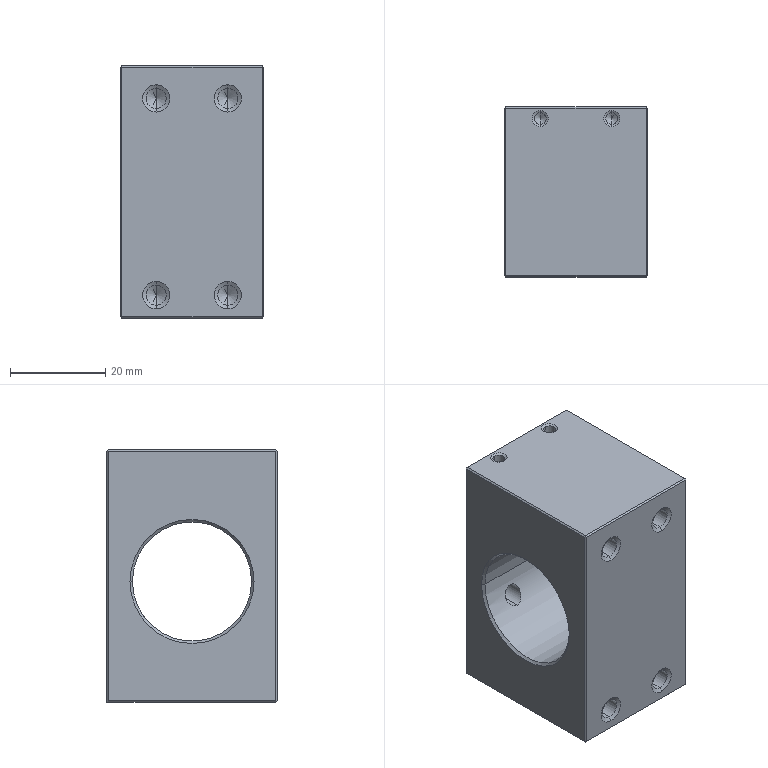Part | NX | 1 solid | 93 faces | box 30 x 35.7 x 53 mm | volume 40484 mm3 | cylinder 38 | cone 38 | plane 17 | commonest cylinder face diameters 4.2 x28 2.5 x8 25 x2